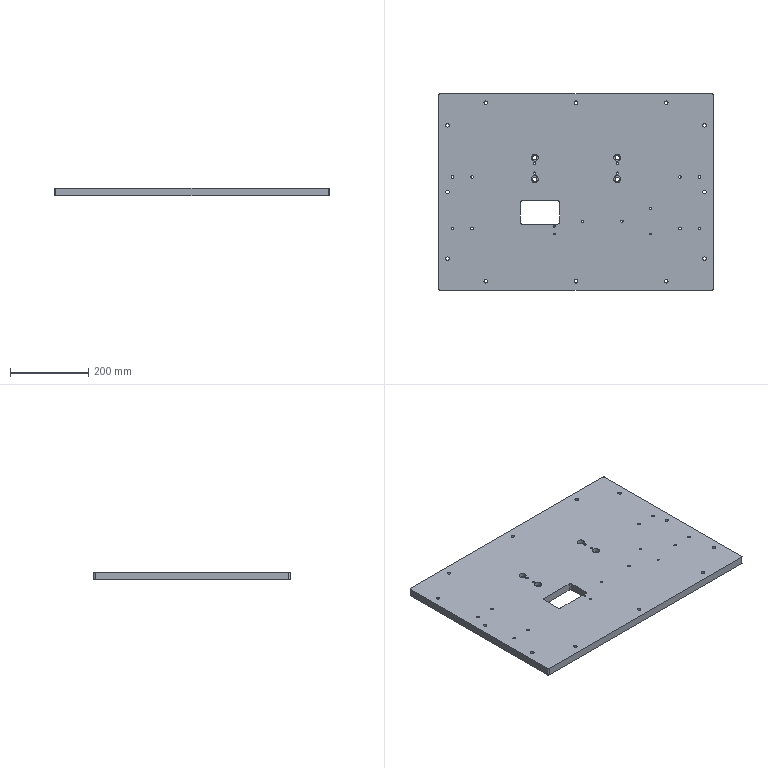Part | STEP file | PN_0004 | 1 solid | 134 faces | box 700 x 500 x 20 mm | volume 6828580 mm3 | cylinder 108 | plane 26 | commonest cylinder face diameters 9 x24 15 x24 6 x16 6.8 x16 5 x8 11 x8